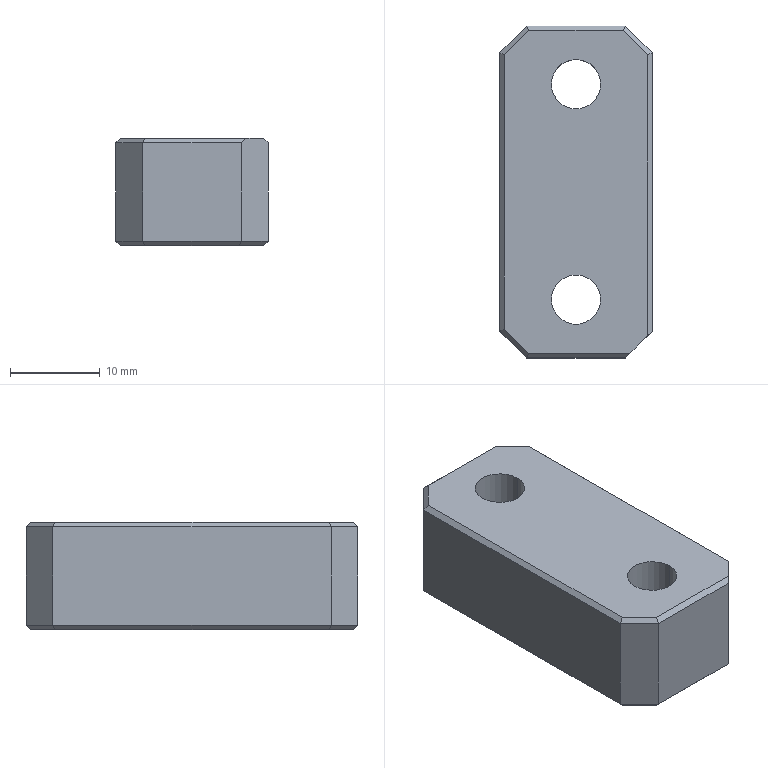Part | Creo | 1 solid | 35 faces | box 17 x 37 x 12 mm | volume 6172 mm3 | plane 27 | cylinder 8 | commonest cylinder face diameters 5.5 x4 9.5 x4
STEP:
#1=CARTESIAN_POINT('',(-82.5,-58.429,-189.));
#2=VERTEX_POINT('',#1);
#3=CARTESIAN_POINT('',(-80.5,-56.429,-189.));
#4=VERTEX_POINT('',#3);
#5=CARTESIAN_POINT('',(-82.5,-58.429,-189.));
#6=DIRECTION('',(0.7071,0.7071,0.));
#7=VECTOR('',#6,2.828);
#8=LINE('',#5,#7);
#9=EDGE_CURVE('',#2,#4,#8,.T.);
#10=ORIENTED_EDGE('',*,*,#9,.F.);
#11=CARTESIAN_POINT('',(-93.793,-58.429,-189.));
#12=VERTEX_POINT('',#11);
#13=CARTESIAN_POINT('',(-82.5,-58.429,-189.));
#14=DIRECTION('',(-1.,0.,0.));
#15=VECTOR('',#14,11.293);
#16=LINE('',#13,#15);
#17=EDGE_CURVE('',#2,#12,#16,.T.);
#18=ORIENTED_EDGE('',*,*,#17,.T.);
#19=CARTESIAN_POINT('',(-96.5,-55.722,-189.));
#20=VERTEX_POINT('',#19);
#21=CARTESIAN_POINT('',(-96.5,-55.722,-189.));
#22=DIRECTION('',(0.7071,-0.7071,0.));
#23=VECTOR('',#22,3.828);
#24=LINE('',#21,#23);
#25=EDGE_CURVE('',#20,#12,#24,.T.);
#26=ORIENTED_EDGE('',*,*,#25,.F.);
#27=CARTESIAN_POINT('',(-96.5,-25.136,-189.));
#28=VERTEX_POINT('',#27);
#29=CARTESIAN_POINT('',(-96.5,-55.722,-189.));
#30=DIRECTION('',(0.,1.,0.));
#31=VECTOR('',#30,30.586);
#32=LINE('',#29,#31);
#33=EDGE_CURVE('',#20,#28,#32,.T.);
#34=ORIENTED_EDGE('',*,*,#33,.T.);
#35=CARTESIAN_POINT('',(-93.793,-22.429,-189.));
#36=VERTEX_POINT('',#35);
#37=CARTESIAN_POINT('',(-93.793,-22.429,-189.));
#38=DIRECTION('',(-0.7071,-0.7071,0.));
#39=VECTOR('',#38,3.828);
#40=LINE('',#37,#39);
#41=EDGE_CURVE('',#36,#28,#40,.T.);
#42=ORIENTED_EDGE('',*,*,#41,.F.);
#43=CARTESIAN_POINT('',(-83.207,-22.429,-189.));
#44=VERTEX_POINT('',#43);
#45=CARTESIAN_POINT('',(-93.793,-22.429,-189.));
#46=DIRECTION('',(1.,0.,0.));
#47=VECTOR('',#46,10.586);
#48=LINE('',#45,#47);
#49=EDGE_CURVE('',#36,#44,#48,.T.);
#50=ORIENTED_EDGE('',*,*,#49,.T.);
#51=CARTESIAN_POINT('',(-80.5,-25.136,-189.));
#52=VERTEX_POINT('',#51);
#53=CARTESIAN_POINT('',(-80.5,-25.136,-189.));
#54=DIRECTION('',(-0.7071,0.7071,0.));
#55=VECTOR('',#54,3.828);
#56=LINE('',#53,#55);
#57=EDGE_CURVE('',#52,#44,#56,.T.);
#58=ORIENTED_EDGE('',*,*,#57,.F.);
#59=CARTESIAN_POINT('',(-80.5,-25.136,-189.));
#60=DIRECTION('',(0.,-1.,0.));
#61=VECTOR('',#60,31.293);
#62=LINE('',#59,#61);
#63=EDGE_CURVE('',#52,#4,#62,.T.);
#64=ORIENTED_EDGE('',*,*,#63,.T.);
#65=EDGE_LOOP('',(#10,#18,#26,#34,#42,#50,#58,#64));
#66=FACE_OUTER_BOUND('',#65,.F.);
#67=CARTESIAN_POINT('',(-85.75,-28.429,-189.));
#68=VERTEX_POINT('',#67);
#69=CARTESIAN_POINT('',(-91.25,-28.429,-189.));
#70=VERTEX_POINT('',#69);
#71=CARTESIAN_POINT('',(-88.5,-28.429,-189.));
#72=DIRECTION('',(0.,0.,-1.));
#73=DIRECTION('',(1.,0.,0.));
#74=AXIS2_PLACEMENT_3D('',#71,#72,#73);
#75=CIRCLE('',#74,2.75);
#76=EDGE_CURVE('',#68,#70,#75,.T.);
#77=ORIENTED_EDGE('',*,*,#76,.F.);
#78=CARTESIAN_POINT('',(-88.5,-28.429,-189.));
#79=DIRECTION('',(0.,0.,-1.));
#80=DIRECTION('',(-1.,0.,0.));
#81=AXIS2_PLACEMENT_3D('',#78,#79,#80);
#82=CIRCLE('',#81,2.75);
#83=EDGE_CURVE('',#70,#68,#82,.T.);
#84=ORIENTED_EDGE('',*,*,#83,.F.);
#85=EDGE_LOOP('',(#77,#84));
#86=FACE_BOUND('',#85,.F.);
#87=CARTESIAN_POINT('',(-85.75,-52.429,-189.));
#88=VERTEX_POINT('',#87);
#89=CARTESIAN_POINT('',(-91.25,-52.429,-189.));
#90=VERTEX_POINT('',#89);
#91=CARTESIAN_POINT('',(-88.5,-52.429,-189.));
#92=DIRECTION('',(0.,0.,-1.));
#93=DIRECTION('',(1.,0.,0.));
#94=AXIS2_PLACEMENT_3D('',#91,#92,#93);
#95=CIRCLE('',#94,2.75);
#96=EDGE_CURVE('',#88,#90,#95,.T.);
#97=ORIENTED_EDGE('',*,*,#96,.F.);
#98=CARTESIAN_POINT('',(-88.5,-52.429,-189.));
#99=DIRECTION('',(0.,0.,-1.));
#100=DIRECTION('',(-1.,0.,0.));
#101=AXIS2_PLACEMENT_3D('',#98,#99,#100);
#102=CIRCLE('',#101,2.75);
#103=EDGE_CURVE('',#90,#88,#102,.T.);
#104=ORIENTED_EDGE('',*,*,#103,.F.);
#105=EDGE_LOOP('',(#97,#104));
#106=FACE_BOUND('',#105,.F.);
#107=CARTESIAN_POINT('',(-88.5,-33.929,-189.));
#108=DIRECTION('',(0.,0.,1.));
#109=DIRECTION('',(-1.,0.,0.));
#110=AXIS2_PLACEMENT_3D('',#107,#108,#109);
#111=PLANE('',#110);
#112=ADVANCED_FACE('',(#66,#86,#106),#111,.T.);
#113=CARTESIAN_POINT('',(-80.,-55.929,-200.5));
#114=VERTEX_POINT('',#113);
#115=CARTESIAN_POINT('',(-80.,-55.929,-189.5));
#116=VERTEX_POINT('',#115);
#117=CARTESIAN_POINT('',(-80.,-55.929,-200.5));
#118=DIRECTION('',(0.,0.,1.));
#119=VECTOR('',#118,11.);
#120=LINE('',#117,#119);
#121=EDGE_CURVE('',#114,#116,#120,.T.);
#122=ORIENTED_EDGE('',*,*,#121,.F.);
#123=CARTESIAN_POINT('',(-83.,-58.929,-200.5));
#124=VERTEX_POINT('',#123);
#125=CARTESIAN_POINT('',(-80.,-55.929,-200.5));
#126=DIRECTION('',(-0.7071,-0.7071,0.));
#127=VECTOR('',#126,4.243);
#128=LINE('',#125,#127);
#129=EDGE_CURVE('',#114,#124,#128,.T.);
#130=ORIENTED_EDGE('',*,*,#129,.T.);
#131=CARTESIAN_POINT('',(-83.,-58.929,-189.5));
#132=VERTEX_POINT('',#131);
#133=CARTESIAN_POINT('',(-83.,-58.929,-189.5));
#134=DIRECTION('',(0.,0.,-1.));
#135=VECTOR('',#134,11.);
#136=LINE('',#133,#135);
#137=EDGE_CURVE('',#132,#124,#136,.T.);
#138=ORIENTED_EDGE('',*,*,#137,.F.);
#139=CARTESIAN_POINT('',(-83.,-58.929,-189.5));
#140=DIRECTION('',(0.5774,0.5774,0.5774));
#141=VECTOR('',#140,0.866);
#142=LINE('',#139,#141);
#143=EDGE_CURVE('',#132,#2,#142,.T.);
#144=ORIENTED_EDGE('',*,*,#143,.T.);
#145=ORIENTED_EDGE('',*,*,#9,.T.);
#146=CARTESIAN_POINT('',(-80.5,-56.429,-189.));
#147=DIRECTION('',(0.5774,0.5774,-0.5774));
#148=VECTOR('',#147,0.866);
#149=LINE('',#146,#148);
#150=EDGE_CURVE('',#4,#116,#149,.T.);
#151=ORIENTED_EDGE('',*,*,#150,.T.);
#152=EDGE_LOOP('',(#122,#130,#138,#144,#145,#151));
#153=FACE_OUTER_BOUND('',#152,.F.);
#154=CARTESIAN_POINT('',(-83.,-58.929,-201.));
#155=DIRECTION('',(-0.7071,0.7071,0.));
#156=DIRECTION('',(0.,0.,-1.));
#157=AXIS2_PLACEMENT_3D('',#154,#155,#156);
#158=PLANE('',#157);
#159=ADVANCED_FACE('',(#153),#158,.F.);
#160=CARTESIAN_POINT('',(-80.,-24.929,-189.5));
#161=VERTEX_POINT('',#160);
#162=CARTESIAN_POINT('',(-80.,-24.929,-200.5));
#163=VERTEX_POINT('',#162);
#164=CARTESIAN_POINT('',(-80.,-24.929,-189.5));
#165=DIRECTION('',(0.,0.,-1.));
#166=VECTOR('',#165,11.);
#167=LINE('',#164,#166);
#168=EDGE_CURVE('',#161,#163,#167,.T.);
#169=ORIENTED_EDGE('',*,*,#168,.T.);
#170=CARTESIAN_POINT('',(-80.,-24.929,-200.5));
#171=DIRECTION('',(0.,-1.,0.));
#172=VECTOR('',#171,31.);
#173=LINE('',#170,#172);
#174=EDGE_CURVE('',#163,#114,#173,.T.);
#175=ORIENTED_EDGE('',*,*,#174,.T.);
#176=ORIENTED_EDGE('',*,*,#121,.T.);
#177=CARTESIAN_POINT('',(-80.,-55.929,-189.5));
#178=DIRECTION('',(0.,1.,0.));
#179=VECTOR('',#178,31.);
#180=LINE('',#177,#179);
#181=EDGE_CURVE('',#116,#161,#180,.T.);
#182=ORIENTED_EDGE('',*,*,#181,.T.);
#183=EDGE_LOOP('',(#169,#175,#176,#182));
#184=FACE_OUTER_BOUND('',#183,.F.);
#185=CARTESIAN_POINT('',(-80.,-33.929,-201.));
#186=DIRECTION('',(1.,0.,0.));
#187=DIRECTION('',(0.,0.,1.));
#188=AXIS2_PLACEMENT_3D('',#185,#186,#187);
#189=PLANE('',#188);
#190=ADVANCED_FACE('',(#184),#189,.T.);
#191=CARTESIAN_POINT('',(-83.,-21.929,-200.5));
#192=VERTEX_POINT('',#191);
#193=CARTESIAN_POINT('',(-83.,-21.929,-189.5));
#194=VERTEX_POINT('',#193);
#195=CARTESIAN_POINT('',(-83.,-21.929,-200.5));
#196=DIRECTION('',(0.,0.,1.));
#197=VECTOR('',#196,11.);
#198=LINE('',#195,#197);
#199=EDGE_CURVE('',#192,#194,#198,.T.);
#200=ORIENTED_EDGE('',*,*,#199,.F.);
#201=CARTESIAN_POINT('',(-83.,-21.929,-200.5));
#202=DIRECTION('',(0.7071,-0.7071,0.));
#203=VECTOR('',#202,4.243);
#204=LINE('',#201,#203);
#205=EDGE_CURVE('',#192,#163,#204,.T.);
#206=ORIENTED_EDGE('',*,*,#205,.T.);
#207=ORIENTED_EDGE('',*,*,#168,.F.);
#208=CARTESIAN_POINT('',(-80.,-24.929,-189.5));
#209=DIRECTION('',(-0.7071,0.7071,0.));
#210=VECTOR('',#209,4.243);
#211=LINE('',#208,#210);
#212=EDGE_CURVE('',#161,#194,#211,.T.);
#213=ORIENTED_EDGE('',*,*,#212,.T.);
#214=EDGE_LOOP('',(#200,#206,#207,#213));
#215=FACE_OUTER_BOUND('',#214,.F.);
#216=CARTESIAN_POINT('',(-80.,-24.929,-201.));
#217=DIRECTION('',(-0.7071,-0.7071,0.));
#218=DIRECTION('',(0.,0.,-1.));
#219=AXIS2_PLACEMENT_3D('',#216,#217,#218);
#220=PLANE('',#219);
#221=ADVANCED_FACE('',(#215),#220,.F.);
#222=ORIENTED_EDGE('',*,*,#199,.T.);
#223=CARTESIAN_POINT('',(-94.,-21.929,-189.5));
#224=VERTEX_POINT('',#223);
#225=CARTESIAN_POINT('',(-83.,-21.929,-189.5));
#226=DIRECTION('',(-1.,0.,0.));
#227=VECTOR('',#226,11.);
#228=LINE('',#225,#227);
#229=EDGE_CURVE('',#194,#224,#228,.T.);
#230=ORIENTED_EDGE('',*,*,#229,.T.);
#231=CARTESIAN_POINT('',(-94.,-21.929,-200.5));
#232=VERTEX_POINT('',#231);
#233=CARTESIAN_POINT('',(-94.,-21.929,-189.5));
#234=DIRECTION('',(0.,0.,-1.));
#235=VECTOR('',#234,11.);
#236=LINE('',#233,#235);
#237=EDGE_CURVE('',#224,#232,#236,.T.);
#238=ORIENTED_EDGE('',*,*,#237,.T.);
#239=CARTESIAN_POINT('',(-94.,-21.929,-200.5));
#240=DIRECTION('',(1.,0.,0.));
#241=VECTOR('',#240,11.);
#242=LINE('',#239,#241);
#243=EDGE_CURVE('',#232,#192,#242,.T.);
#244=ORIENTED_EDGE('',*,*,#243,.T.);
#245=EDGE_LOOP('',(#222,#230,#238,#244));
#246=FACE_OUTER_BOUND('',#245,.F.);
#247=CARTESIAN_POINT('',(-88.5,-21.929,-201.));
#248=DIRECTION('',(0.,1.,0.));
#249=DIRECTION('',(0.,0.,-1.));
#250=AXIS2_PLACEMENT_3D('',#247,#248,#249);
#251=PLANE('',#250);
#252=ADVANCED_FACE('',(#246),#251,.T.);
#253=CARTESIAN_POINT('',(-93.793,-22.429,-189.));
#254=DIRECTION('',(-0.2811,0.6786,-0.6786));
#255=VECTOR('',#254,0.7368);
#256=LINE('',#253,#255);
#257=EDGE_CURVE('',#36,#224,#256,.T.);
#258=ORIENTED_EDGE('',*,*,#257,.T.);
#259=ORIENTED_EDGE('',*,*,#229,.F.);
#260=CARTESIAN_POINT('',(-83.207,-22.429,-189.));
#261=DIRECTION('',(0.2811,0.6786,-0.6786));
#262=VECTOR('',#261,0.7368);
#263=LINE('',#260,#262);
#264=EDGE_CURVE('',#44,#194,#263,.T.);
#265=ORIENTED_EDGE('',*,*,#264,.F.);
#266=ORIENTED_EDGE('',*,*,#49,.F.);
#267=EDGE_LOOP('',(#258,#259,#265,#266));
#268=FACE_OUTER_BOUND('',#267,.F.);
#269=CARTESIAN_POINT('',(-88.5,-21.929,-189.5));
#270=DIRECTION('',(0.,-0.7071,-0.7071));
#271=DIRECTION('',(1.,0.,0.));
#272=AXIS2_PLACEMENT_3D('',#269,#270,#271);
#273=PLANE('',#272);
#274=ADVANCED_FACE('',(#268),#273,.F.);
#275=CARTESIAN_POINT('',(-97.,-24.929,-189.5));
#276=VERTEX_POINT('',#275);
#277=CARTESIAN_POINT('',(-96.5,-25.136,-189.));
#278=DIRECTION('',(-0.6786,0.2811,-0.6786));
#279=VECTOR('',#278,0.7368);
#280=LINE('',#277,#279);
#281=EDGE_CURVE('',#28,#276,#280,.T.);
#282=ORIENTED_EDGE('',*,*,#281,.T.);
#283=CARTESIAN_POINT('',(-94.,-21.929,-189.5));
#284=DIRECTION('',(-0.7071,-0.7071,0.));
#285=VECTOR('',#284,4.243);
#286=LINE('',#283,#285);
#287=EDGE_CURVE('',#224,#276,#286,.T.);
#288=ORIENTED_EDGE('',*,*,#287,.F.);
#289=ORIENTED_EDGE('',*,*,#257,.F.);
#290=ORIENTED_EDGE('',*,*,#41,.T.);
#291=EDGE_LOOP('',(#282,#288,#289,#290));
#292=FACE_OUTER_BOUND('',#291,.F.);
#293=CARTESIAN_POINT('',(-96.896,-25.533,-189.));
#294=DIRECTION('',(-0.5,0.5,0.7071));
#295=DIRECTION('',(0.7071,0.7071,0.));
#296=AXIS2_PLACEMENT_3D('',#293,#294,#295);
#297=PLANE('',#296);
#298=ADVANCED_FACE('',(#292),#297,.T.);
#299=CARTESIAN_POINT('',(-97.,-55.929,-189.5));
#300=VERTEX_POINT('',#299);
#301=CARTESIAN_POINT('',(-96.5,-55.722,-189.));
#302=DIRECTION('',(-0.6786,-0.2811,-0.6786));
#303=VECTOR('',#302,0.7368);
#304=LINE('',#301,#303);
#305=EDGE_CURVE('',#20,#300,#304,.T.);
#306=ORIENTED_EDGE('',*,*,#305,.T.);
#307=CARTESIAN_POINT('',(-97.,-24.929,-189.5));
#308=DIRECTION('',(0.,-1.,0.));
#309=VECTOR('',#308,31.);
#310=LINE('',#307,#309);
#311=EDGE_CURVE('',#276,#300,#310,.T.);
#312=ORIENTED_EDGE('',*,*,#311,.F.);
#313=ORIENTED_EDGE('',*,*,#281,.F.);
#314=ORIENTED_EDGE('',*,*,#33,.F.);
#315=EDGE_LOOP('',(#306,#312,#313,#314));
#316=FACE_OUTER_BOUND('',#315,.F.);
#317=CARTESIAN_POINT('',(-97.,-33.929,-189.5));
#318=DIRECTION('',(0.7071,0.,-0.7071));
#319=DIRECTION('',(0.,1.,0.));
#320=AXIS2_PLACEMENT_3D('',#317,#318,#319);
#321=PLANE('',#320);
#322=ADVANCED_FACE('',(#316),#321,.F.);
#323=CARTESIAN_POINT('',(-94.,-58.929,-189.5));
#324=VERTEX_POINT('',#323);
#325=CARTESIAN_POINT('',(-93.793,-58.429,-189.));
#326=DIRECTION('',(-0.2811,-0.6786,-0.6786));
#327=VECTOR('',#326,0.7368);
#328=LINE('',#325,#327);
#329=EDGE_CURVE('',#12,#324,#328,.T.);
#330=ORIENTED_EDGE('',*,*,#329,.T.);
#331=CARTESIAN_POINT('',(-97.,-55.929,-189.5));
#332=DIRECTION('',(0.7071,-0.7071,0.));
#333=VECTOR('',#332,4.243);
#334=LINE('',#331,#333);
#335=EDGE_CURVE('',#300,#324,#334,.T.);
#336=ORIENTED_EDGE('',*,*,#335,.F.);
#337=ORIENTED_EDGE('',*,*,#305,.F.);
#338=ORIENTED_EDGE('',*,*,#25,.T.);
#339=EDGE_LOOP('',(#330,#336,#337,#338));
#340=FACE_OUTER_BOUND('',#339,.F.);
#341=CARTESIAN_POINT('',(-103.396,-48.826,-189.));
#342=DIRECTION('',(-0.5,-0.5,0.7071));
#343=DIRECTION('',(-0.7071,0.7071,0.));
#344=AXIS2_PLACEMENT_3D('',#341,#342,#343);
#345=PLANE('',#344);
#346=ADVANCED_FACE('',(#340),#345,.T.);
#347=ORIENTED_EDGE('',*,*,#143,.F.);
#348=CARTESIAN_POINT('',(-94.,-58.929,-189.5));
#349=DIRECTION('',(1.,0.,0.));
#350=VECTOR('',#349,11.);
#351=LINE('',#348,#350);
#352=EDGE_CURVE('',#324,#132,#351,.T.);
#353=ORIENTED_EDGE('',*,*,#352,.F.);
#354=ORIENTED_EDGE('',*,*,#329,.F.);
#355=ORIENTED_EDGE('',*,*,#17,.F.);
#356=EDGE_LOOP('',(#347,#353,#354,#355));
#357=FACE_OUTER_BOUND('',#356,.F.);
#358=CARTESIAN_POINT('',(-88.5,-58.929,-189.5));
#359=DIRECTION('',(0.,0.7071,-0.7071));
#360=DIRECTION('',(-1.,0.,0.));
#361=AXIS2_PLACEMENT_3D('',#358,#359,#360);
#362=PLANE('',#361);
#363=ADVANCED_FACE('',(#357),#362,.F.);
#364=ORIENTED_EDGE('',*,*,#137,.T.);
#365=CARTESIAN_POINT('',(-94.,-58.929,-200.5));
#366=VERTEX_POINT('',#365);
#367=CARTESIAN_POINT('',(-83.,-58.929,-200.5));
#368=DIRECTION('',(-1.,0.,0.));
#369=VECTOR('',#368,11.);
#370=LINE('',#367,#369);
#371=EDGE_CURVE('',#124,#366,#370,.T.);
#372=ORIENTED_EDGE('',*,*,#371,.T.);
#373=CARTESIAN_POINT('',(-94.,-58.929,-200.5));
#374=DIRECTION('',(0.,0.,1.));
#375=VECTOR('',#374,11.);
#376=LINE('',#373,#375);
#377=EDGE_CURVE('',#366,#324,#376,.T.);
#378=ORIENTED_EDGE('',*,*,#377,.T.);
#379=ORIENTED_EDGE('',*,*,#352,.T.);
#380=EDGE_LOOP('',(#364,#372,#378,#379));
#381=FACE_OUTER_BOUND('',#380,.F.);
#382=CARTESIAN_POINT('',(-88.5,-58.929,-201.));
#383=DIRECTION('',(0.,-1.,0.));
#384=DIRECTION('',(0.,0.,1.));
#385=AXIS2_PLACEMENT_3D('',#382,#383,#384);
#386=PLANE('',#385);
#387=ADVANCED_FACE('',(#381),#386,.T.);
#388=CARTESIAN_POINT('',(-93.793,-58.429,-201.));
#389=VERTEX_POINT('',#388);
#390=CARTESIAN_POINT('',(-93.793,-58.429,-201.));
#391=DIRECTION('',(-0.2811,-0.6786,0.6786));
#392=VECTOR('',#391,0.7368);
#393=LINE('',#390,#392);
#394=EDGE_CURVE('',#389,#366,#393,.T.);
#395=ORIENTED_EDGE('',*,*,#394,.T.);
#396=ORIENTED_EDGE('',*,*,#371,.F.);
#397=CARTESIAN_POINT('',(-83.207,-58.429,-201.));
#398=VERTEX_POINT('',#397);
#399=CARTESIAN_POINT('',(-83.207,-58.429,-201.));
#400=DIRECTION('',(0.2811,-0.6786,0.6786));
#401=VECTOR('',#400,0.7368);
#402=LINE('',#399,#401);
#403=EDGE_CURVE('',#398,#124,#402,.T.);
#404=ORIENTED_EDGE('',*,*,#403,.F.);
#405=CARTESIAN_POINT('',(-93.793,-58.429,-201.));
#406=DIRECTION('',(1.,0.,0.));
#407=VECTOR('',#406,10.586);
#408=LINE('',#405,#407);
#409=EDGE_CURVE('',#389,#398,#408,.T.);
#410=ORIENTED_EDGE('',*,*,#409,.F.);
#411=EDGE_LOOP('',(#395,#396,#404,#410));
#412=FACE_OUTER_BOUND('',#411,.F.);
#413=CARTESIAN_POINT('',(-88.5,-58.929,-200.5));
#414=DIRECTION('',(0.,0.7071,0.7071));
#415=DIRECTION('',(1.,0.,0.));
#416=AXIS2_PLACEMENT_3D('',#413,#414,#415);
#417=PLANE('',#416);
#418=ADVANCED_FACE('',(#412),#417,.F.);
#419=ORIENTED_EDGE('',*,*,#394,.F.);
#420=CARTESIAN_POINT('',(-96.5,-55.722,-201.));
#421=VERTEX_POINT('',#420);
#422=CARTESIAN_POINT('',(-93.793,-58.429,-201.));
#423=DIRECTION('',(-0.7071,0.7071,0.));
#424=VECTOR('',#423,3.828);
#425=LINE('',#422,#424);
#426=EDGE_CURVE('',#389,#421,#425,.T.);
#427=ORIENTED_EDGE('',*,*,#426,.T.);
#428=CARTESIAN_POINT('',(-97.,-55.929,-200.5));
#429=VERTEX_POINT('',#428);
#430=CARTESIAN_POINT('',(-97.,-55.929,-200.5));
#431=DIRECTION('',(0.6786,0.2811,-0.6786));
#432=VECTOR('',#431,0.7368);
#433=LINE('',#430,#432);
#434=EDGE_CURVE('',#429,#421,#433,.T.);
#435=ORIENTED_EDGE('',*,*,#434,.F.);
#436=CARTESIAN_POINT('',(-94.,-58.929,-200.5));
#437=DIRECTION('',(-0.7071,0.7071,0.));
#438=VECTOR('',#437,4.243);
#439=LINE('',#436,#438);
#440=EDGE_CURVE('',#366,#429,#439,.T.);
#441=ORIENTED_EDGE('',*,*,#440,.F.);
#442=EDGE_LOOP('',(#419,#427,#435,#441));
#443=FACE_OUTER_BOUND('',#442,.F.);
#444=CARTESIAN_POINT('',(-103.396,-48.826,-201.));
#445=DIRECTION('',(-0.5,-0.5,-0.7071));
#446=DIRECTION('',(0.7071,-0.7071,0.));
#447=AXIS2_PLACEMENT_3D('',#444,#445,#446);
#448=PLANE('',#447);
#449=ADVANCED_FACE('',(#443),#448,.T.);
#450=CARTESIAN_POINT('',(-83.207,-22.429,-201.));
#451=VERTEX_POINT('',#450);
#452=CARTESIAN_POINT('',(-93.793,-22.429,-201.));
#453=VERTEX_POINT('',#452);
#454=CARTESIAN_POINT('',(-83.207,-22.429,-201.));
#455=DIRECTION('',(-1.,0.,0.));
#456=VECTOR('',#455,10.586);
#457=LINE('',#454,#456);
#458=EDGE_CURVE('',#451,#453,#457,.T.);
#459=ORIENTED_EDGE('',*,*,#458,.T.);
#460=CARTESIAN_POINT('',(-96.5,-25.136,-201.));
#461=VERTEX_POINT('',#460);
#462=CARTESIAN_POINT('',(-96.5,-25.136,-201.));
#463=DIRECTION('',(0.7071,0.7071,0.));
#464=VECTOR('',#463,3.828);
#465=LINE('',#462,#464);
#466=EDGE_CURVE('',#461,#453,#465,.T.);
#467=ORIENTED_EDGE('',*,*,#466,.F.);
#468=CARTESIAN_POINT('',(-96.5,-25.136,-201.));
#469=DIRECTION('',(0.,-1.,0.));
#470=VECTOR('',#469,30.586);
#471=LINE('',#468,#470);
#472=EDGE_CURVE('',#461,#421,#471,.T.);
#473=ORIENTED_EDGE('',*,*,#472,.T.);
#474=ORIENTED_EDGE('',*,*,#426,.F.);
#475=ORIENTED_EDGE('',*,*,#409,.T.);
#476=CARTESIAN_POINT('',(-80.5,-55.722,-201.));
#477=VERTEX_POINT('',#476);
#478=CARTESIAN_POINT('',(-80.5,-55.722,-201.));
#479=DIRECTION('',(-0.7071,-0.7071,0.));
#480=VECTOR('',#479,3.828);
#481=LINE('',#478,#480);
#482=EDGE_CURVE('',#477,#398,#481,.T.);
#483=ORIENTED_EDGE('',*,*,#482,.F.);
#484=CARTESIAN_POINT('',(-80.5,-25.136,-201.));
#485=VERTEX_POINT('',#484);
#486=CARTESIAN_POINT('',(-80.5,-55.722,-201.));
#487=DIRECTION('',(0.,1.,0.));
#488=VECTOR('',#487,30.586);
#489=LINE('',#486,#488);
#490=EDGE_CURVE('',#477,#485,#489,.T.);
#491=ORIENTED_EDGE('',*,*,#490,.T.);
#492=CARTESIAN_POINT('',(-83.207,-22.429,-201.));
#493=DIRECTION('',(0.7071,-0.7071,0.));
#494=VECTOR('',#493,3.828);
#495=LINE('',#492,#494);
#496=EDGE_CURVE('',#451,#485,#495,.T.);
#497=ORIENTED_EDGE('',*,*,#496,.F.);
#498=EDGE_LOOP('',(#459,#467,#473,#474,#475,#483,#491,#497));
#499=FACE_OUTER_BOUND('',#498,.F.);
#500=CARTESIAN_POINT('',(-93.25,-52.429,-201.));
#501=VERTEX_POINT('',#500);
#502=CARTESIAN_POINT('',(-83.75,-52.429,-201.));
#503=VERTEX_POINT('',#502);
#504=CARTESIAN_POINT('',(-88.5,-52.429,-201.));
#505=DIRECTION('',(0.,0.,1.));
#506=DIRECTION('',(-1.,0.,0.));
#507=AXIS2_PLACEMENT_3D('',#504,#505,#506);
#508=CIRCLE('',#507,4.75);
#509=EDGE_CURVE('',#501,#503,#508,.T.);
#510=ORIENTED_EDGE('',*,*,#509,.F.);
#511=CARTESIAN_POINT('',(-88.5,-52.429,-201.));
#512=DIRECTION('',(0.,0.,1.));
#513=DIRECTION('',(1.,0.,0.));
#514=AXIS2_PLACEMENT_3D('',#511,#512,#513);
#515=CIRCLE('',#514,4.75);
#516=EDGE_CURVE('',#503,#501,#515,.T.);
#517=ORIENTED_EDGE('',*,*,#516,.F.);
#518=EDGE_LOOP('',(#510,#517));
#519=FACE_BOUND('',#518,.F.);
#520=CARTESIAN_POINT('',(-93.25,-28.429,-201.));
#521=VERTEX_POINT('',#520);
#522=CARTESIAN_POINT('',(-83.75,-28.429,-201.));
#523=VERTEX_POINT('',#522);
#524=CARTESIAN_POINT('',(-88.5,-28.429,-201.));
#525=DIRECTION('',(0.,0.,1.));
#526=DIRECTION('',(-1.,0.,0.));
#527=AXIS2_PLACEMENT_3D('',#524,#525,#526);
#528=CIRCLE('',#527,4.75);
#529=EDGE_CURVE('',#521,#523,#528,.T.);
#530=ORIENTED_EDGE('',*,*,#529,.F.);
#531=CARTESIAN_POINT('',(-88.5,-28.429,-201.));
#532=DIRECTION('',(0.,0.,1.));
#533=DIRECTION('',(1.,0.,0.));
#534=AXIS2_PLACEMENT_3D('',#531,#532,#533);
#535=CIRCLE('',#534,4.75);
#536=EDGE_CURVE('',#523,#521,#535,.T.);
#537=ORIENTED_EDGE('',*,*,#536,.F.);
#538=EDGE_LOOP('',(#530,#537));
#539=FACE_BOUND('',#538,.F.);
#540=CARTESIAN_POINT('',(-88.5,-33.929,-201.));
#541=DIRECTION('',(0.,0.,-1.));
#542=DIRECTION('',(1.,0.,0.));
#543=AXIS2_PLACEMENT_3D('',#540,#541,#542);
#544=PLANE('',#543);
#545=ADVANCED_FACE('',(#499,#519,#539),#544,.T.);
#546=CARTESIAN_POINT('',(-94.,-21.929,-200.5));
#547=DIRECTION('',(0.2811,-0.6786,-0.6786));
#548=VECTOR('',#547,0.7368);
#549=LINE('',#546,#548);
#550=EDGE_CURVE('',#232,#453,#549,.T.);
#551=ORIENTED_EDGE('',*,*,#550,.T.);
#552=ORIENTED_EDGE('',*,*,#458,.F.);
#553=CARTESIAN_POINT('',(-83.,-21.929,-200.5));
#554=DIRECTION('',(-0.2811,-0.6786,-0.6786));
#555=VECTOR('',#554,0.7368);
#556=LINE('',#553,#555);
#557=EDGE_CURVE('',#192,#451,#556,.T.);
#558=ORIENTED_EDGE('',*,*,#557,.F.);
#559=ORIENTED_EDGE('',*,*,#243,.F.);
#560=EDGE_LOOP('',(#551,#552,#558,#559));
#561=FACE_OUTER_BOUND('',#560,.F.);
#562=CARTESIAN_POINT('',(-88.5,-21.929,-200.5));
#563=DIRECTION('',(0.,-0.7071,0.7071));
#564=DIRECTION('',(-1.,0.,0.));
#565=AXIS2_PLACEMENT_3D('',#562,#563,#564);
#566=PLANE('',#565);
#567=ADVANCED_FACE('',(#561),#566,.F.);
#568=CARTESIAN_POINT('',(-97.,-24.929,-200.5));
#569=VERTEX_POINT('',#568);
#570=CARTESIAN_POINT('',(-97.,-24.929,-200.5));
#571=DIRECTION('',(0.6786,-0.2811,-0.6786));
#572=VECTOR('',#571,0.7368);
#573=LINE('',#570,#572);
#574=EDGE_CURVE('',#569,#461,#573,.T.);
#575=ORIENTED_EDGE('',*,*,#574,.T.);
#576=ORIENTED_EDGE('',*,*,#466,.T.);
#577=ORIENTED_EDGE('',*,*,#550,.F.);
#578=CARTESIAN_POINT('',(-97.,-24.929,-200.5));
#579=DIRECTION('',(0.7071,0.7071,0.));
#580=VECTOR('',#579,4.243);
#581=LINE('',#578,#580);
#582=EDGE_CURVE('',#569,#232,#581,.T.);
#583=ORIENTED_EDGE('',*,*,#582,.F.);
#584=EDGE_LOOP('',(#575,#576,#577,#583));
#585=FACE_OUTER_BOUND('',#584,.F.);
#586=CARTESIAN_POINT('',(-96.896,-25.533,-201.));
#587=DIRECTION('',(-0.5,0.5,-0.7071));
#588=DIRECTION('',(-0.7071,-0.7071,0.));
#589=AXIS2_PLACEMENT_3D('',#586,#587,#588);
#590=PLANE('',#589);
#591=ADVANCED_FACE('',(#585),#590,.T.);
#592=ORIENTED_EDGE('',*,*,#434,.T.);
#593=ORIENTED_EDGE('',*,*,#472,.F.);
#594=ORIENTED_EDGE('',*,*,#574,.F.);
#595=CARTESIAN_POINT('',(-97.,-55.929,-200.5));
#596=DIRECTION('',(0.,1.,0.));
#597=VECTOR('',#596,31.);
#598=LINE('',#595,#597);
#599=EDGE_CURVE('',#429,#569,#598,.T.);
#600=ORIENTED_EDGE('',*,*,#599,.F.);
#601=EDGE_LOOP('',(#592,#593,#594,#600));
#602=FACE_OUTER_BOUND('',#601,.F.);
#603=CARTESIAN_POINT('',(-97.,-33.929,-200.5));
#604=DIRECTION('',(0.7071,0.,0.7071));
#605=DIRECTION('',(0.,-1.,0.));
#606=AXIS2_PLACEMENT_3D('',#603,#604,#605);
#607=PLANE('',#606);
#608=ADVANCED_FACE('',(#602),#607,.F.);
#609=CARTESIAN_POINT('',(-97.,-55.929,-189.5));
#610=DIRECTION('',(0.,0.,-1.));
#611=VECTOR('',#610,11.);
#612=LINE('',#609,#611);
#613=EDGE_CURVE('',#300,#429,#612,.T.);
#614=ORIENTED_EDGE('',*,*,#613,.T.);
#615=ORIENTED_EDGE('',*,*,#599,.T.);
#616=CARTESIAN_POINT('',(-97.,-24.929,-200.5));
#617=DIRECTION('',(0.,0.,1.));
#618=VECTOR('',#617,11.);
#619=LINE('',#616,#618);
#620=EDGE_CURVE('',#569,#276,#619,.T.);
#621=ORIENTED_EDGE('',*,*,#620,.T.);
#622=ORIENTED_EDGE('',*,*,#311,.T.);
#623=EDGE_LOOP('',(#614,#615,#621,#622));
#624=FACE_OUTER_BOUND('',#623,.F.);
#625=CARTESIAN_POINT('',(-97.,-33.929,-201.));
#626=DIRECTION('',(-1.,0.,0.));
#627=DIRECTION('',(0.,0.,-1.));
#628=AXIS2_PLACEMENT_3D('',#625,#626,#627);
#629=PLANE('',#628);
#630=ADVANCED_FACE('',(#624),#629,.T.);
#631=ORIENTED_EDGE('',*,*,#377,.F.);
#632=ORIENTED_EDGE('',*,*,#440,.T.);
#633=ORIENTED_EDGE('',*,*,#613,.F.);
#634=ORIENTED_EDGE('',*,*,#335,.T.);
#635=EDGE_LOOP('',(#631,#632,#633,#634));
#636=FACE_OUTER_BOUND('',#635,.F.);
#637=CARTESIAN_POINT('',(-97.,-55.929,-201.));
#638=DIRECTION('',(0.7071,0.7071,0.));
#639=DIRECTION('',(0.,0.,-1.));
#640=AXIS2_PLACEMENT_3D('',#637,#638,#639);
#641=PLANE('',#640);
#642=ADVANCED_FACE('',(#636),#641,.F.);
#643=ORIENTED_EDGE('',*,*,#237,.F.);
#644=ORIENTED_EDGE('',*,*,#287,.T.);
#645=ORIENTED_EDGE('',*,*,#620,.F.);
#646=ORIENTED_EDGE('',*,*,#582,.T.);
#647=EDGE_LOOP('',(#643,#644,#645,#646));
#648=FACE_OUTER_BOUND('',#647,.F.);
#649=CARTESIAN_POINT('',(-94.,-21.929,-201.));
#650=DIRECTION('',(0.7071,-0.7071,0.));
#651=DIRECTION('',(0.,0.,-1.));
#652=AXIS2_PLACEMENT_3D('',#649,#650,#651);
#653=PLANE('',#652);
#654=ADVANCED_FACE('',(#648),#653,.F.);
#655=ORIENTED_EDGE('',*,*,#557,.T.);
#656=ORIENTED_EDGE('',*,*,#496,.T.);
#657=CARTESIAN_POINT('',(-80.5,-25.136,-201.));
#658=DIRECTION('',(0.6786,0.2811,0.6786));
#659=VECTOR('',#658,0.7368);
#660=LINE('',#657,#659);
#661=EDGE_CURVE('',#485,#163,#660,.T.);
#662=ORIENTED_EDGE('',*,*,#661,.T.);
#663=ORIENTED_EDGE('',*,*,#205,.F.);
#664=EDGE_LOOP('',(#655,#656,#662,#663));
#665=FACE_OUTER_BOUND('',#664,.F.);
#666=CARTESIAN_POINT('',(-80.104,-25.533,-201.));
#667=DIRECTION('',(0.5,0.5,-0.7071));
#668=DIRECTION('',(-0.7071,0.7071,0.));
#669=AXIS2_PLACEMENT_3D('',#666,#667,#668);
#670=PLANE('',#669);
#671=ADVANCED_FACE('',(#665),#670,.T.);
#672=CARTESIAN_POINT('',(-80.5,-55.722,-201.));
#673=DIRECTION('',(0.6786,-0.2811,0.6786));
#674=VECTOR('',#673,0.7368);
#675=LINE('',#672,#674);
#676=EDGE_CURVE('',#477,#114,#675,.T.);
#677=ORIENTED_EDGE('',*,*,#676,.T.);
#678=ORIENTED_EDGE('',*,*,#174,.F.);
#679=ORIENTED_EDGE('',*,*,#661,.F.);
#680=ORIENTED_EDGE('',*,*,#490,.F.);
#681=EDGE_LOOP('',(#677,#678,#679,#680));
#682=FACE_OUTER_BOUND('',#681,.F.);
#683=CARTESIAN_POINT('',(-80.,-33.929,-200.5));
#684=DIRECTION('',(-0.7071,0.,0.7071));
#685=DIRECTION('',(0.,1.,0.));
#686=AXIS2_PLACEMENT_3D('',#683,#684,#685);
#687=PLANE('',#686);
#688=ADVANCED_FACE('',(#682),#687,.F.);
#689=ORIENTED_EDGE('',*,*,#403,.T.);
#690=ORIENTED_EDGE('',*,*,#129,.F.);
#691=ORIENTED_EDGE('',*,*,#676,.F.);
#692=ORIENTED_EDGE('',*,*,#482,.T.);
#693=EDGE_LOOP('',(#689,#690,#691,#692));
#694=FACE_OUTER_BOUND('',#693,.F.);
#695=CARTESIAN_POINT('',(-73.604,-48.826,-201.));
#696=DIRECTION('',(0.5,-0.5,-0.7071));
#697=DIRECTION('',(0.7071,0.7071,0.));
#698=AXIS2_PLACEMENT_3D('',#695,#696,#697);
#699=PLANE('',#698);
#700=ADVANCED_FACE('',(#694),#699,.T.);
#701=CARTESIAN_POINT('',(-83.75,-52.429,-195.));
#702=VERTEX_POINT('',#701);
#703=CARTESIAN_POINT('',(-93.25,-52.429,-195.));
#704=VERTEX_POINT('',#703);
#705=CARTESIAN_POINT('',(-88.5,-52.429,-195.));
#706=DIRECTION('',(0.,0.,-1.));
#707=DIRECTION('',(1.,0.,0.));
#708=AXIS2_PLACEMENT_3D('',#705,#706,#707);
#709=CIRCLE('',#708,4.75);
#710=EDGE_CURVE('',#702,#704,#709,.T.);
#711=ORIENTED_EDGE('',*,*,#710,.T.);
#712=CARTESIAN_POINT('',(-93.25,-52.429,-195.));
#713=DIRECTION('',(0.,0.,-1.));
#714=VECTOR('',#713,6.);
#715=LINE('',#712,#714);
#716=EDGE_CURVE('',#704,#501,#715,.T.);
#717=ORIENTED_EDGE('',*,*,#716,.T.);
#718=ORIENTED_EDGE('',*,*,#509,.T.);
#719=CARTESIAN_POINT('',(-83.75,-52.429,-195.));
#720=DIRECTION('',(0.,0.,-1.));
#721=VECTOR('',#720,6.);
#722=LINE('',#719,#721);
#723=EDGE_CURVE('',#702,#503,#722,.T.);
#724=ORIENTED_EDGE('',*,*,#723,.F.);
#725=EDGE_LOOP('',(#711,#717,#718,#724));
#726=FACE_OUTER_BOUND('',#725,.F.);
#727=CARTESIAN_POINT('',(-88.5,-52.429,-201.));
#728=DIRECTION('',(0.,0.,-1.));
#729=DIRECTION('',(1.,0.,0.));
#730=AXIS2_PLACEMENT_3D('',#727,#728,#729);
#731=CYLINDRICAL_SURFACE('',#730,4.75);
#732=ADVANCED_FACE('',(#726),#731,.F.);
#733=CARTESIAN_POINT('',(-88.5,-52.429,-195.));
#734=DIRECTION('',(0.,0.,-1.));
#735=DIRECTION('',(-1.,0.,0.));
#736=AXIS2_PLACEMENT_3D('',#733,#734,#735);
#737=CIRCLE('',#736,4.75);
#738=EDGE_CURVE('',#704,#702,#737,.T.);
#739=ORIENTED_EDGE('',*,*,#738,.F.);
#740=ORIENTED_EDGE('',*,*,#710,.F.);
#741=EDGE_LOOP('',(#739,#740));
#742=FACE_OUTER_BOUND('',#741,.F.);
#743=CARTESIAN_POINT('',(-91.25,-52.429,-195.));
#744=VERTEX_POINT('',#743);
#745=CARTESIAN_POINT('',(-85.75,-52.429,-195.));
#746=VERTEX_POINT('',#745);
#747=CARTESIAN_POINT('',(-88.5,-52.429,-195.));
#748=DIRECTION('',(0.,0.,1.));
#749=DIRECTION('',(-1.,0.,0.));
#750=AXIS2_PLACEMENT_3D('',#747,#748,#749);
#751=CIRCLE('',#750,2.75);
#752=EDGE_CURVE('',#744,#746,#751,.T.);
#753=ORIENTED_EDGE('',*,*,#752,.F.);
#754=CARTESIAN_POINT('',(-88.5,-52.429,-195.));
#755=DIRECTION('',(0.,0.,1.));
#756=DIRECTION('',(1.,0.,0.));
#757=AXIS2_PLACEMENT_3D('',#754,#755,#756);
#758=CIRCLE('',#757,2.75);
#759=EDGE_CURVE('',#746,#744,#758,.T.);
#760=ORIENTED_EDGE('',*,*,#759,.F.);
#761=EDGE_LOOP('',(#753,#760));
#762=FACE_BOUND('',#761,.F.);
#763=CARTESIAN_POINT('',(-88.5,-47.679,-195.));
#764=DIRECTION('',(0.,0.,1.));
#765=DIRECTION('',(-1.,0.,0.));
#766=AXIS2_PLACEMENT_3D('',#763,#764,#765);
#767=PLANE('',#766);
#768=ADVANCED_FACE('',(#742,#762),#767,.F.);
#769=ORIENTED_EDGE('',*,*,#96,.T.);
#770=CARTESIAN_POINT('',(-91.25,-52.429,-189.));
#771=DIRECTION('',(0.,0.,-1.));
#772=VECTOR('',#771,6.);
#773=LINE('',#770,#772);
#774=EDGE_CURVE('',#90,#744,#773,.T.);
#775=ORIENTED_EDGE('',*,*,#774,.T.);
#776=ORIENTED_EDGE('',*,*,#752,.T.);
#777=CARTESIAN_POINT('',(-85.75,-52.429,-189.));
#778=DIRECTION('',(0.,0.,-1.));
#779=VECTOR('',#778,6.);
#780=LINE('',#777,#779);
#781=EDGE_CURVE('',#88,#746,#780,.T.);
#782=ORIENTED_EDGE('',*,*,#781,.F.);
#783=EDGE_LOOP('',(#769,#775,#776,#782));
#784=FACE_OUTER_BOUND('',#783,.F.);
#785=CARTESIAN_POINT('',(-88.5,-52.429,-201.));
#786=DIRECTION('',(0.,0.,-1.));
#787=DIRECTION('',(1.,0.,0.));
#788=AXIS2_PLACEMENT_3D('',#785,#786,#787);
#789=CYLINDRICAL_SURFACE('',#788,2.75);
#790=ADVANCED_FACE('',(#784),#789,.F.);
#791=ORIENTED_EDGE('',*,*,#103,.T.);
#792=ORIENTED_EDGE('',*,*,#781,.T.);
#793=ORIENTED_EDGE('',*,*,#759,.T.);
#794=ORIENTED_EDGE('',*,*,#774,.F.);
#795=EDGE_LOOP('',(#791,#792,#793,#794));
#796=FACE_OUTER_BOUND('',#795,.F.);
#797=CARTESIAN_POINT('',(-88.5,-52.429,-201.));
#798=DIRECTION('',(0.,0.,-1.));
#799=DIRECTION('',(1.,0.,0.));
#800=AXIS2_PLACEMENT_3D('',#797,#798,#799);
#801=CYLINDRICAL_SURFACE('',#800,2.75);
#802=ADVANCED_FACE('',(#796),#801,.F.);
#803=ORIENTED_EDGE('',*,*,#738,.T.);
#804=ORIENTED_EDGE('',*,*,#723,.T.);
#805=ORIENTED_EDGE('',*,*,#516,.T.);
#806=ORIENTED_EDGE('',*,*,#716,.F.);
#807=EDGE_LOOP('',(#803,#804,#805,#806));
#808=FACE_OUTER_BOUND('',#807,.F.);
#809=CARTESIAN_POINT('',(-88.5,-52.429,-201.));
#810=DIRECTION('',(0.,0.,-1.));
#811=DIRECTION('',(1.,0.,0.));
#812=AXIS2_PLACEMENT_3D('',#809,#810,#811);
#813=CYLINDRICAL_SURFACE('',#812,4.75);
#814=ADVANCED_FACE('',(#808),#813,.F.);
#815=CARTESIAN_POINT('',(-83.75,-28.429,-195.));
#816=VERTEX_POINT('',#815);
#817=CARTESIAN_POINT('',(-93.25,-28.429,-195.));
#818=VERTEX_POINT('',#817);
#819=CARTESIAN_POINT('',(-88.5,-28.429,-195.));
#820=DIRECTION('',(0.,0.,-1.));
#821=DIRECTION('',(1.,0.,0.));
#822=AXIS2_PLACEMENT_3D('',#819,#820,#821);
#823=CIRCLE('',#822,4.75);
#824=EDGE_CURVE('',#816,#818,#823,.T.);
#825=ORIENTED_EDGE('',*,*,#824,.T.);
#826=CARTESIAN_POINT('',(-93.25,-28.429,-195.));
#827=DIRECTION('',(0.,0.,-1.));
#828=VECTOR('',#827,6.);
#829=LINE('',#826,#828);
#830=EDGE_CURVE('',#818,#521,#829,.T.);
#831=ORIENTED_EDGE('',*,*,#830,.T.);
#832=ORIENTED_EDGE('',*,*,#529,.T.);
#833=CARTESIAN_POINT('',(-83.75,-28.429,-195.));
#834=DIRECTION('',(0.,0.,-1.));
#835=VECTOR('',#834,6.);
#836=LINE('',#833,#835);
#837=EDGE_CURVE('',#816,#523,#836,.T.);
#838=ORIENTED_EDGE('',*,*,#837,.F.);
#839=EDGE_LOOP('',(#825,#831,#832,#838));
#840=FACE_OUTER_BOUND('',#839,.F.);
#841=CARTESIAN_POINT('',(-88.5,-28.429,-201.));
#842=DIRECTION('',(0.,0.,-1.));
#843=DIRECTION('',(1.,0.,0.));
#844=AXIS2_PLACEMENT_3D('',#841,#842,#843);
#845=CYLINDRICAL_SURFACE('',#844,4.75);
#846=ADVANCED_FACE('',(#840),#845,.F.);
#847=CARTESIAN_POINT('',(-88.5,-28.429,-195.));
#848=DIRECTION('',(0.,0.,-1.));
#849=DIRECTION('',(-1.,0.,0.));
#850=AXIS2_PLACEMENT_3D('',#847,#848,#849);
#851=CIRCLE('',#850,4.75);
#852=EDGE_CURVE('',#818,#816,#851,.T.);
#853=ORIENTED_EDGE('',*,*,#852,.F.);
#854=ORIENTED_EDGE('',*,*,#824,.F.);
#855=EDGE_LOOP('',(#853,#854));
#856=FACE_OUTER_BOUND('',#855,.F.);
#857=CARTESIAN_POINT('',(-91.25,-28.429,-195.));
#858=VERTEX_POINT('',#857);
#859=CARTESIAN_POINT('',(-85.75,-28.429,-195.));
#860=VERTEX_POINT('',#859);
#861=CARTESIAN_POINT('',(-88.5,-28.429,-195.));
#862=DIRECTION('',(0.,0.,1.));
#863=DIRECTION('',(-1.,0.,0.));
#864=AXIS2_PLACEMENT_3D('',#861,#862,#863);
#865=CIRCLE('',#864,2.75);
#866=EDGE_CURVE('',#858,#860,#865,.T.);
#867=ORIENTED_EDGE('',*,*,#866,.F.);
#868=CARTESIAN_POINT('',(-88.5,-28.429,-195.));
#869=DIRECTION('',(0.,0.,1.));
#870=DIRECTION('',(1.,0.,0.));
#871=AXIS2_PLACEMENT_3D('',#868,#869,#870);
#872=CIRCLE('',#871,2.75);
#873=EDGE_CURVE('',#860,#858,#872,.T.);
#874=ORIENTED_EDGE('',*,*,#873,.F.);
#875=EDGE_LOOP('',(#867,#874));
#876=FACE_BOUND('',#875,.F.);
#877=CARTESIAN_POINT('',(-88.5,-23.679,-195.));
#878=DIRECTION('',(0.,0.,1.));
#879=DIRECTION('',(-1.,0.,0.));
#880=AXIS2_PLACEMENT_3D('',#877,#878,#879);
#881=PLANE('',#880);
#882=ADVANCED_FACE('',(#856,#876),#881,.F.);
#883=ORIENTED_EDGE('',*,*,#76,.T.);
#884=CARTESIAN_POINT('',(-91.25,-28.429,-189.));
#885=DIRECTION('',(0.,0.,-1.));
#886=VECTOR('',#885,6.);
#887=LINE('',#884,#886);
#888=EDGE_CURVE('',#70,#858,#887,.T.);
#889=ORIENTED_EDGE('',*,*,#888,.T.);
#890=ORIENTED_EDGE('',*,*,#866,.T.);
#891=CARTESIAN_POINT('',(-85.75,-28.429,-189.));
#892=DIRECTION('',(0.,0.,-1.));
#893=VECTOR('',#892,6.);
#894=LINE('',#891,#893);
#895=EDGE_CURVE('',#68,#860,#894,.T.);
#896=ORIENTED_EDGE('',*,*,#895,.F.);
#897=EDGE_LOOP('',(#883,#889,#890,#896));
#898=FACE_OUTER_BOUND('',#897,.F.);
#899=CARTESIAN_POINT('',(-88.5,-28.429,-201.));
#900=DIRECTION('',(0.,0.,-1.));
#901=DIRECTION('',(1.,0.,0.));
#902=AXIS2_PLACEMENT_3D('',#899,#900,#901);
#903=CYLINDRICAL_SURFACE('',#902,2.75);
#904=ADVANCED_FACE('',(#898),#903,.F.);
#905=ORIENTED_EDGE('',*,*,#83,.T.);
#906=ORIENTED_EDGE('',*,*,#895,.T.);
#907=ORIENTED_EDGE('',*,*,#873,.T.);
#908=ORIENTED_EDGE('',*,*,#888,.F.);
#909=EDGE_LOOP('',(#905,#906,#907,#908));
#910=FACE_OUTER_BOUND('',#909,.F.);
#911=CARTESIAN_POINT('',(-88.5,-28.429,-201.));
#912=DIRECTION('',(0.,0.,-1.));
#913=DIRECTION('',(1.,0.,0.));
#914=AXIS2_PLACEMENT_3D('',#911,#912,#913);
#915=CYLINDRICAL_SURFACE('',#914,2.75);
#916=ADVANCED_FACE('',(#910),#915,.F.);
#917=ORIENTED_EDGE('',*,*,#852,.T.);
#918=ORIENTED_EDGE('',*,*,#837,.T.);
#919=ORIENTED_EDGE('',*,*,#536,.T.);
#920=ORIENTED_EDGE('',*,*,#830,.F.);
#921=EDGE_LOOP('',(#917,#918,#919,#920));
#922=FACE_OUTER_BOUND('',#921,.F.);
#923=CARTESIAN_POINT('',(-88.5,-28.429,-201.));
#924=DIRECTION('',(0.,0.,-1.));
#925=DIRECTION('',(1.,0.,0.));
#926=AXIS2_PLACEMENT_3D('',#923,#924,#925);
#927=CYLINDRICAL_SURFACE('',#926,4.75);
#928=ADVANCED_FACE('',(#922),#927,.F.);
#929=ORIENTED_EDGE('',*,*,#264,.T.);
#930=ORIENTED_EDGE('',*,*,#212,.F.);
#931=CARTESIAN_POINT('',(-80.5,-25.136,-189.));
#932=DIRECTION('',(0.6786,0.2811,-0.6786));
#933=VECTOR('',#932,0.7368);
#934=LINE('',#931,#933);
#935=EDGE_CURVE('',#52,#161,#934,.T.);
#936=ORIENTED_EDGE('',*,*,#935,.F.);
#937=ORIENTED_EDGE('',*,*,#57,.T.);
#938=EDGE_LOOP('',(#929,#930,#936,#937));
#939=FACE_OUTER_BOUND('',#938,.F.);
#940=CARTESIAN_POINT('',(-80.104,-25.533,-189.));
#941=DIRECTION('',(0.5,0.5,0.7071));
#942=DIRECTION('',(0.7071,-0.7071,0.));
#943=AXIS2_PLACEMENT_3D('',#940,#941,#942);
#944=PLANE('',#943);
#945=ADVANCED_FACE('',(#939),#944,.T.);
#946=ORIENTED_EDGE('',*,*,#935,.T.);
#947=ORIENTED_EDGE('',*,*,#181,.F.);
#948=ORIENTED_EDGE('',*,*,#150,.F.);
#949=ORIENTED_EDGE('',*,*,#63,.F.);
#950=EDGE_LOOP('',(#946,#947,#948,#949));
#951=FACE_OUTER_BOUND('',#950,.F.);
#952=CARTESIAN_POINT('',(-80.,-33.929,-189.5));
#953=DIRECTION('',(-0.7071,0.,-0.7071));
#954=DIRECTION('',(0.,-1.,0.));
#955=AXIS2_PLACEMENT_3D('',#952,#953,#954);
#956=PLANE('',#955);
#957=ADVANCED_FACE('',(#951),#956,.F.);
#958=CLOSED_SHELL('',(#112,#159,#190,#221,#252,#274,#298,#322,#346,#363,#387,#418,#449,#545,#567,#591,#608,#630,#642,#654,#671,#688,#700,#732,#768,#790,#802,#814,#846,#882,#904,#916,#928,#945,#957));
#959=MANIFOLD_SOLID_BREP('',#958);
#960=(LENGTH_UNIT()NAMED_UNIT(*)SI_UNIT(.MILLI.,.METRE.));
#961=UNCERTAINTY_MEASURE_WITH_UNIT(LENGTH_MEASURE(0.004245),#960,'','');
#962=(NAMED_UNIT(*)PLANE_ANGLE_UNIT()SI_UNIT($,.RADIAN.));
#963=PLANE_ANGLE_MEASURE_WITH_UNIT(PLANE_ANGLE_MEASURE(0.01745),#962);
#964=(CONVERSION_BASED_UNIT('DEGREE',#963)NAMED_UNIT(*)PLANE_ANGLE_UNIT());
#965=(NAMED_UNIT(*)SI_UNIT($,.STERADIAN.)SOLID_ANGLE_UNIT());
#966=(GEOMETRIC_REPRESENTATION_CONTEXT(3)GLOBAL_UNCERTAINTY_ASSIGNED_CONTEXT((#961))GLOBAL_UNIT_ASSIGNED_CONTEXT((#960,#964,#965))REPRESENTATION_CONTEXT('',''));
#967=ADVANCED_BREP_SHAPE_REPRESENTATION('',(#959),#966);